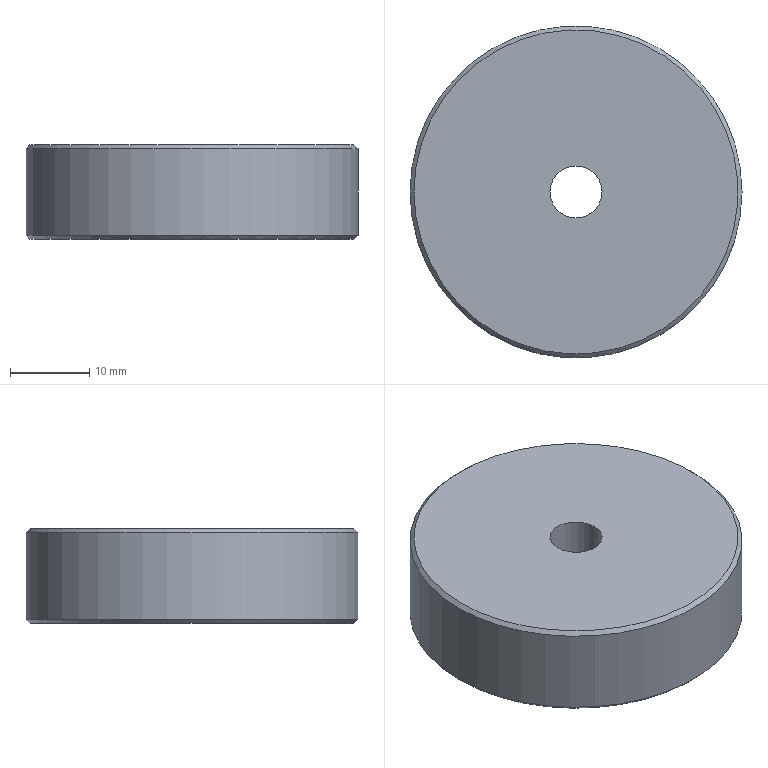Part | STEP file | solid 207 | 1 solid | 8 faces | box 42 x 42 x 12 mm | volume 15756 mm3 | plane 3 | cylinder 3 | cone 2 | commonest cylinder face diameters 6.6 x1 11 x1 42 x1